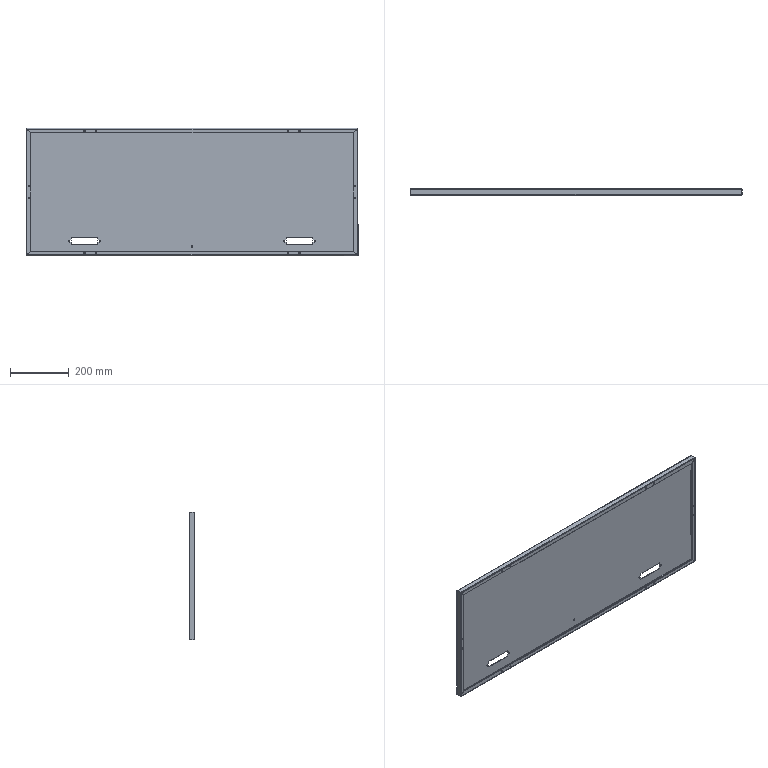Part | STEP file | JBJ-P-1000-11 | 1 solid | 107 faces | box 1135 x 20 x 435 mm | volume 703191 mm3 | plane 58 | cylinder 33 | spline 16 | commonest cylinder face diameters 4 x12 2 x8 4.4 x8 7 x4 6.5 x1